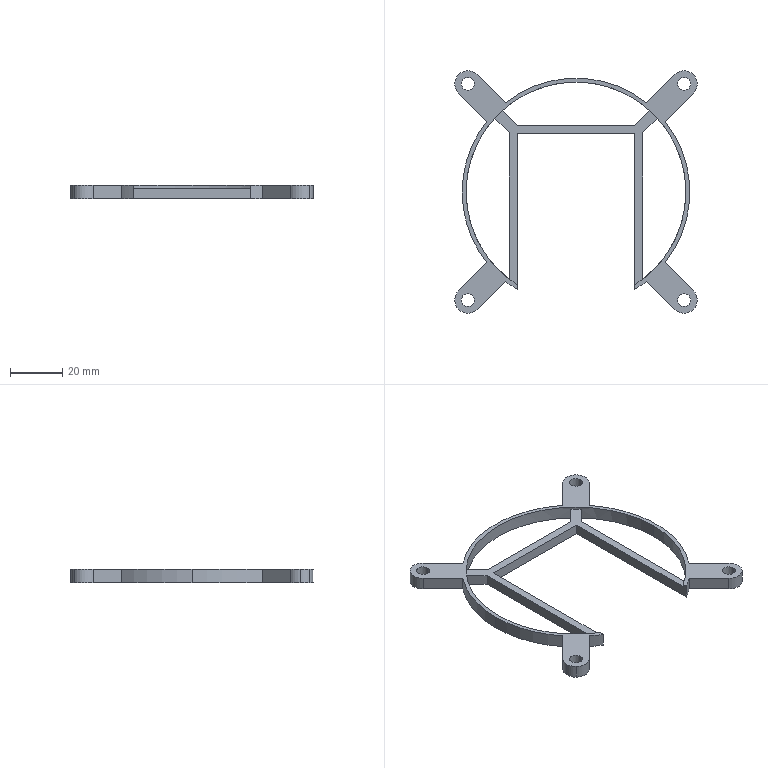Part | SolidWorks | features ICE 4, CirPattern 1, Extrusion 1, Fillet 1 | 1 solid | 48 faces | box 92.873 x 92.873 x 5 mm | volume 7282 mm3 | cylinder 27 | plane 21 | commonest cylinder face diameters 10 x10 5 x8 87.2 x6 84.2 x3